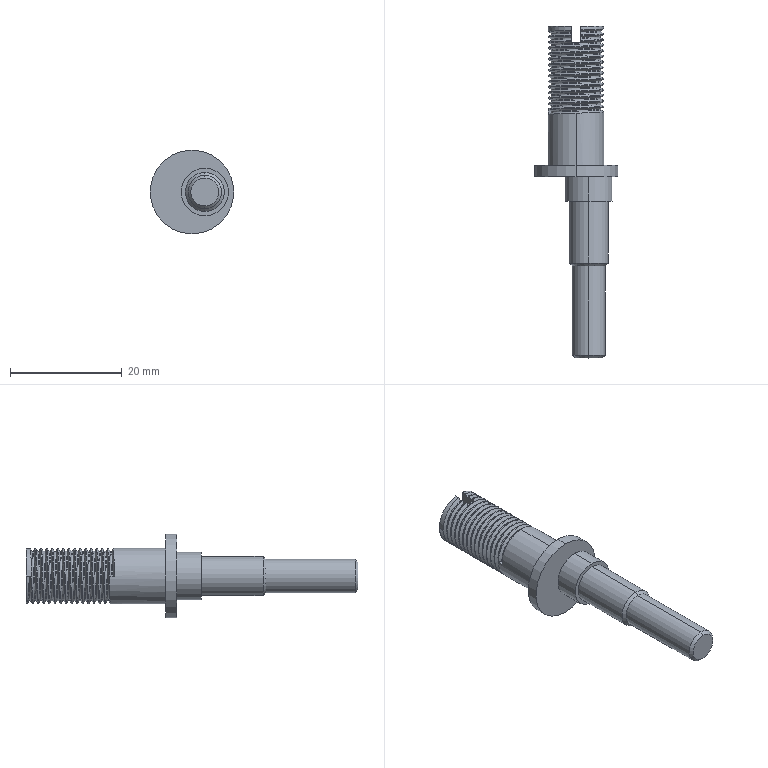Part | SolidWorks | features ICE 5, Chamfer 2, Extrusion 1, SweepThread 1 | 1 solid | 72 faces | box 15 x 59.5 x 15 mm | volume 3289 mm3 | cylinder 40 | spline 17 | plane 11 | cone 4 | commonest cylinder face diameters 10 x32 6 x2 7 x2 8.5 x2 15 x2